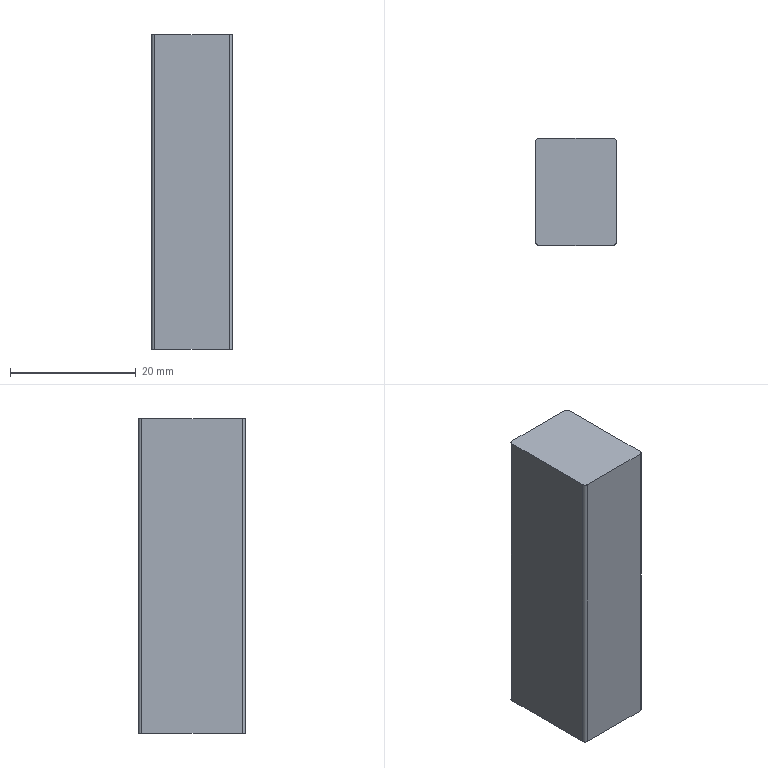Part | NX | features BREP 1 | 1 solid | 10 faces | box 12.887 x 16.955 x 50 mm | volume 10914 mm3 | plane 6 | cylinder 4 | commonest cylinder face diameters 1 x4
STEP:
#1=CARTESIAN_POINT('',(-5.944,8.477,-40.6));
#2=VERTEX_POINT('',#1);
#3=CARTESIAN_POINT('',(-6.444,7.978,-40.6));
#4=VERTEX_POINT('',#3);
#5=CARTESIAN_POINT('',(-5.944,7.978,-40.6));
#6=DIRECTION('',(0.,0.,1.));
#7=DIRECTION('',(1.,0.,0.));
#8=AXIS2_PLACEMENT_3D('',#5,#6,#7);
#9=CIRCLE('',#8,0.5);
#10=EDGE_CURVE('',#2,#4,#9,.T.);
#11=ORIENTED_EDGE('',*,*,#10,.F.);
#12=CARTESIAN_POINT('',(-5.944,8.477,-90.6));
#13=VERTEX_POINT('',#12);
#14=CARTESIAN_POINT('',(-5.944,8.477,-90.6));
#15=DIRECTION('',(0.,0.,1.));
#16=VECTOR('',#15,1000.);
#17=LINE('',#14,#16);
#18=EDGE_CURVE('',#13,#2,#17,.T.);
#19=ORIENTED_EDGE('',*,*,#18,.F.);
#20=CARTESIAN_POINT('',(-6.444,7.978,-90.6));
#21=VERTEX_POINT('',#20);
#22=CARTESIAN_POINT('',(-5.944,7.978,-90.6));
#23=DIRECTION('',(0.,0.,1.));
#24=DIRECTION('',(1.,0.,0.));
#25=AXIS2_PLACEMENT_3D('',#22,#23,#24);
#26=CIRCLE('',#25,0.5);
#27=EDGE_CURVE('',#13,#21,#26,.T.);
#28=ORIENTED_EDGE('',*,*,#27,.T.);
#29=CARTESIAN_POINT('',(-6.444,7.978,-90.6));
#30=DIRECTION('',(0.,0.,1.));
#31=VECTOR('',#30,1000.);
#32=LINE('',#29,#31);
#33=EDGE_CURVE('',#21,#4,#32,.T.);
#34=ORIENTED_EDGE('',*,*,#33,.T.);
#35=EDGE_LOOP('',(#11,#19,#28,#34));
#36=FACE_BOUND('',#35,.T.);
#37=CARTESIAN_POINT('',(-5.944,7.978,-90.6));
#38=DIRECTION('',(0.,0.,1.));
#39=DIRECTION('',(-1.,0.,0.));
#40=AXIS2_PLACEMENT_3D('',#37,#38,#39);
#41=CYLINDRICAL_SURFACE('',#40,0.5);
#42=ADVANCED_FACE('',(#36),#41,.T.);
#43=CARTESIAN_POINT('',(-6.444,-7.977,-40.6));
#44=VERTEX_POINT('',#43);
#45=CARTESIAN_POINT('',(-6.444,-7.977,-40.6));
#46=DIRECTION('',(0.,1.,0.));
#47=VECTOR('',#46,1000.);
#48=LINE('',#45,#47);
#49=EDGE_CURVE('',#44,#4,#48,.T.);
#50=ORIENTED_EDGE('',*,*,#49,.T.);
#51=ORIENTED_EDGE('',*,*,#33,.F.);
#52=CARTESIAN_POINT('',(-6.444,-7.977,-90.6));
#53=VERTEX_POINT('',#52);
#54=CARTESIAN_POINT('',(-6.444,-7.977,-90.6));
#55=DIRECTION('',(0.,1.,0.));
#56=VECTOR('',#55,1000.);
#57=LINE('',#54,#56);
#58=EDGE_CURVE('',#53,#21,#57,.T.);
#59=ORIENTED_EDGE('',*,*,#58,.F.);
#60=CARTESIAN_POINT('',(-6.444,-7.977,-90.6));
#61=DIRECTION('',(0.,0.,1.));
#62=VECTOR('',#61,1000.);
#63=LINE('',#60,#62);
#64=EDGE_CURVE('',#53,#44,#63,.T.);
#65=ORIENTED_EDGE('',*,*,#64,.T.);
#66=EDGE_LOOP('',(#50,#51,#59,#65));
#67=FACE_BOUND('',#66,.T.);
#68=CARTESIAN_POINT('',(-6.444,-7.977,-90.6));
#69=DIRECTION('',(1.,0.,0.));
#70=DIRECTION('',(0.,-1.,0.));
#71=AXIS2_PLACEMENT_3D('',#68,#69,#70);
#72=PLANE('',#71);
#73=ADVANCED_FACE('',(#67),#72,.F.);
#74=CARTESIAN_POINT('',(-5.944,-8.477,-40.6));
#75=VERTEX_POINT('',#74);
#76=CARTESIAN_POINT('',(-5.944,-7.977,-40.6));
#77=DIRECTION('',(0.,0.,1.));
#78=DIRECTION('',(1.,0.,0.));
#79=AXIS2_PLACEMENT_3D('',#76,#77,#78);
#80=CIRCLE('',#79,0.5);
#81=EDGE_CURVE('',#44,#75,#80,.T.);
#82=ORIENTED_EDGE('',*,*,#81,.F.);
#83=ORIENTED_EDGE('',*,*,#64,.F.);
#84=CARTESIAN_POINT('',(-5.944,-8.477,-90.6));
#85=VERTEX_POINT('',#84);
#86=CARTESIAN_POINT('',(-5.944,-7.977,-90.6));
#87=DIRECTION('',(0.,0.,1.));
#88=DIRECTION('',(1.,0.,0.));
#89=AXIS2_PLACEMENT_3D('',#86,#87,#88);
#90=CIRCLE('',#89,0.5);
#91=EDGE_CURVE('',#53,#85,#90,.T.);
#92=ORIENTED_EDGE('',*,*,#91,.T.);
#93=CARTESIAN_POINT('',(-5.944,-8.477,-90.6));
#94=DIRECTION('',(0.,0.,1.));
#95=VECTOR('',#94,1000.);
#96=LINE('',#93,#95);
#97=EDGE_CURVE('',#85,#75,#96,.T.);
#98=ORIENTED_EDGE('',*,*,#97,.T.);
#99=EDGE_LOOP('',(#82,#83,#92,#98));
#100=FACE_BOUND('',#99,.T.);
#101=CARTESIAN_POINT('',(-5.944,-7.977,-90.6));
#102=DIRECTION('',(0.,0.,1.));
#103=DIRECTION('',(-1.,0.,0.));
#104=AXIS2_PLACEMENT_3D('',#101,#102,#103);
#105=CYLINDRICAL_SURFACE('',#104,0.5);
#106=ADVANCED_FACE('',(#100),#105,.T.);
#107=CARTESIAN_POINT('',(5.944,-8.477,-40.6));
#108=VERTEX_POINT('',#107);
#109=CARTESIAN_POINT('',(5.944,-8.477,-40.6));
#110=DIRECTION('',(-1.,0.,0.));
#111=VECTOR('',#110,1000.);
#112=LINE('',#109,#111);
#113=EDGE_CURVE('',#108,#75,#112,.T.);
#114=ORIENTED_EDGE('',*,*,#113,.T.);
#115=ORIENTED_EDGE('',*,*,#97,.F.);
#116=CARTESIAN_POINT('',(5.944,-8.477,-90.6));
#117=VERTEX_POINT('',#116);
#118=CARTESIAN_POINT('',(5.944,-8.477,-90.6));
#119=DIRECTION('',(-1.,0.,0.));
#120=VECTOR('',#119,1000.);
#121=LINE('',#118,#120);
#122=EDGE_CURVE('',#117,#85,#121,.T.);
#123=ORIENTED_EDGE('',*,*,#122,.F.);
#124=CARTESIAN_POINT('',(5.944,-8.477,-90.6));
#125=DIRECTION('',(0.,0.,1.));
#126=VECTOR('',#125,1000.);
#127=LINE('',#124,#126);
#128=EDGE_CURVE('',#117,#108,#127,.T.);
#129=ORIENTED_EDGE('',*,*,#128,.T.);
#130=EDGE_LOOP('',(#114,#115,#123,#129));
#131=FACE_BOUND('',#130,.T.);
#132=CARTESIAN_POINT('',(5.944,-8.477,-90.6));
#133=DIRECTION('',(0.,1.,0.));
#134=DIRECTION('',(0.,0.,-1.));
#135=AXIS2_PLACEMENT_3D('',#132,#133,#134);
#136=PLANE('',#135);
#137=ADVANCED_FACE('',(#131),#136,.F.);
#138=CARTESIAN_POINT('',(6.444,-7.977,-40.6));
#139=VERTEX_POINT('',#138);
#140=CARTESIAN_POINT('',(5.944,-7.977,-40.6));
#141=DIRECTION('',(0.,0.,1.));
#142=DIRECTION('',(1.,0.,0.));
#143=AXIS2_PLACEMENT_3D('',#140,#141,#142);
#144=CIRCLE('',#143,0.5);
#145=EDGE_CURVE('',#108,#139,#144,.T.);
#146=ORIENTED_EDGE('',*,*,#145,.F.);
#147=ORIENTED_EDGE('',*,*,#128,.F.);
#148=CARTESIAN_POINT('',(6.444,-7.977,-90.6));
#149=VERTEX_POINT('',#148);
#150=CARTESIAN_POINT('',(5.944,-7.977,-90.6));
#151=DIRECTION('',(0.,0.,1.));
#152=DIRECTION('',(1.,0.,0.));
#153=AXIS2_PLACEMENT_3D('',#150,#151,#152);
#154=CIRCLE('',#153,0.5);
#155=EDGE_CURVE('',#117,#149,#154,.T.);
#156=ORIENTED_EDGE('',*,*,#155,.T.);
#157=CARTESIAN_POINT('',(6.444,-7.977,-90.6));
#158=DIRECTION('',(0.,0.,1.));
#159=VECTOR('',#158,1000.);
#160=LINE('',#157,#159);
#161=EDGE_CURVE('',#149,#139,#160,.T.);
#162=ORIENTED_EDGE('',*,*,#161,.T.);
#163=EDGE_LOOP('',(#146,#147,#156,#162));
#164=FACE_BOUND('',#163,.T.);
#165=CARTESIAN_POINT('',(5.944,-7.977,-90.6));
#166=DIRECTION('',(0.,0.,1.));
#167=DIRECTION('',(-1.,0.,0.));
#168=AXIS2_PLACEMENT_3D('',#165,#166,#167);
#169=CYLINDRICAL_SURFACE('',#168,0.5);
#170=ADVANCED_FACE('',(#164),#169,.T.);
#171=CARTESIAN_POINT('',(6.444,7.978,-40.6));
#172=VERTEX_POINT('',#171);
#173=CARTESIAN_POINT('',(6.444,7.978,-40.6));
#174=DIRECTION('',(0.,-1.,0.));
#175=VECTOR('',#174,1000.);
#176=LINE('',#173,#175);
#177=EDGE_CURVE('',#172,#139,#176,.T.);
#178=ORIENTED_EDGE('',*,*,#177,.T.);
#179=ORIENTED_EDGE('',*,*,#161,.F.);
#180=CARTESIAN_POINT('',(6.444,7.978,-90.6));
#181=VERTEX_POINT('',#180);
#182=CARTESIAN_POINT('',(6.444,7.978,-90.6));
#183=DIRECTION('',(0.,-1.,0.));
#184=VECTOR('',#183,1000.);
#185=LINE('',#182,#184);
#186=EDGE_CURVE('',#181,#149,#185,.T.);
#187=ORIENTED_EDGE('',*,*,#186,.F.);
#188=CARTESIAN_POINT('',(6.444,7.978,-90.6));
#189=DIRECTION('',(0.,0.,1.));
#190=VECTOR('',#189,1000.);
#191=LINE('',#188,#190);
#192=EDGE_CURVE('',#181,#172,#191,.T.);
#193=ORIENTED_EDGE('',*,*,#192,.T.);
#194=EDGE_LOOP('',(#178,#179,#187,#193));
#195=FACE_BOUND('',#194,.T.);
#196=CARTESIAN_POINT('',(6.444,7.978,-90.6));
#197=DIRECTION('',(-1.,0.,0.));
#198=DIRECTION('',(0.,0.,-1.));
#199=AXIS2_PLACEMENT_3D('',#196,#197,#198);
#200=PLANE('',#199);
#201=ADVANCED_FACE('',(#195),#200,.F.);
#202=CARTESIAN_POINT('',(5.944,8.477,-40.6));
#203=VERTEX_POINT('',#202);
#204=CARTESIAN_POINT('',(5.944,7.978,-40.6));
#205=DIRECTION('',(0.,0.,1.));
#206=DIRECTION('',(1.,0.,0.));
#207=AXIS2_PLACEMENT_3D('',#204,#205,#206);
#208=CIRCLE('',#207,0.5);
#209=EDGE_CURVE('',#172,#203,#208,.T.);
#210=ORIENTED_EDGE('',*,*,#209,.F.);
#211=ORIENTED_EDGE('',*,*,#192,.F.);
#212=CARTESIAN_POINT('',(5.944,8.477,-90.6));
#213=VERTEX_POINT('',#212);
#214=CARTESIAN_POINT('',(5.944,7.978,-90.6));
#215=DIRECTION('',(0.,0.,1.));
#216=DIRECTION('',(1.,0.,0.));
#217=AXIS2_PLACEMENT_3D('',#214,#215,#216);
#218=CIRCLE('',#217,0.5);
#219=EDGE_CURVE('',#181,#213,#218,.T.);
#220=ORIENTED_EDGE('',*,*,#219,.T.);
#221=CARTESIAN_POINT('',(5.944,8.477,-90.6));
#222=DIRECTION('',(0.,0.,1.));
#223=VECTOR('',#222,1000.);
#224=LINE('',#221,#223);
#225=EDGE_CURVE('',#213,#203,#224,.T.);
#226=ORIENTED_EDGE('',*,*,#225,.T.);
#227=EDGE_LOOP('',(#210,#211,#220,#226));
#228=FACE_BOUND('',#227,.T.);
#229=CARTESIAN_POINT('',(5.944,7.978,-90.6));
#230=DIRECTION('',(0.,0.,1.));
#231=DIRECTION('',(-1.,0.,0.));
#232=AXIS2_PLACEMENT_3D('',#229,#230,#231);
#233=CYLINDRICAL_SURFACE('',#232,0.5);
#234=ADVANCED_FACE('',(#228),#233,.T.);
#235=CARTESIAN_POINT('',(-5.944,8.477,-40.6));
#236=DIRECTION('',(1.,0.,0.));
#237=VECTOR('',#236,1000.);
#238=LINE('',#235,#237);
#239=EDGE_CURVE('',#2,#203,#238,.T.);
#240=ORIENTED_EDGE('',*,*,#239,.T.);
#241=ORIENTED_EDGE('',*,*,#225,.F.);
#242=CARTESIAN_POINT('',(-5.944,8.477,-90.6));
#243=DIRECTION('',(1.,0.,0.));
#244=VECTOR('',#243,1000.);
#245=LINE('',#242,#244);
#246=EDGE_CURVE('',#13,#213,#245,.T.);
#247=ORIENTED_EDGE('',*,*,#246,.F.);
#248=ORIENTED_EDGE('',*,*,#18,.T.);
#249=EDGE_LOOP('',(#240,#241,#247,#248));
#250=FACE_BOUND('',#249,.T.);
#251=CARTESIAN_POINT('',(-5.944,8.477,-90.6));
#252=DIRECTION('',(0.,-1.,0.));
#253=DIRECTION('',(-1.,0.,0.));
#254=AXIS2_PLACEMENT_3D('',#251,#252,#253);
#255=PLANE('',#254);
#256=ADVANCED_FACE('',(#250),#255,.F.);
#257=ORIENTED_EDGE('',*,*,#27,.F.);
#258=ORIENTED_EDGE('',*,*,#246,.T.);
#259=ORIENTED_EDGE('',*,*,#219,.F.);
#260=ORIENTED_EDGE('',*,*,#186,.T.);
#261=ORIENTED_EDGE('',*,*,#155,.F.);
#262=ORIENTED_EDGE('',*,*,#122,.T.);
#263=ORIENTED_EDGE('',*,*,#91,.F.);
#264=ORIENTED_EDGE('',*,*,#58,.T.);
#265=EDGE_LOOP('',(#257,#258,#259,#260,#261,#262,#263,#264));
#266=FACE_BOUND('',#265,.T.);
#267=CARTESIAN_POINT('',(-5.944,7.978,-90.6));
#268=DIRECTION('',(0.,0.,1.));
#269=DIRECTION('',(-1.,0.,0.));
#270=AXIS2_PLACEMENT_3D('',#267,#268,#269);
#271=PLANE('',#270);
#272=ADVANCED_FACE('',(#266),#271,.F.);
#273=ORIENTED_EDGE('',*,*,#10,.T.);
#274=ORIENTED_EDGE('',*,*,#49,.F.);
#275=ORIENTED_EDGE('',*,*,#81,.T.);
#276=ORIENTED_EDGE('',*,*,#113,.F.);
#277=ORIENTED_EDGE('',*,*,#145,.T.);
#278=ORIENTED_EDGE('',*,*,#177,.F.);
#279=ORIENTED_EDGE('',*,*,#209,.T.);
#280=ORIENTED_EDGE('',*,*,#239,.F.);
#281=EDGE_LOOP('',(#273,#274,#275,#276,#277,#278,#279,#280));
#282=FACE_BOUND('',#281,.T.);
#283=CARTESIAN_POINT('',(-5.944,7.978,-40.6));
#284=DIRECTION('',(0.,0.,1.));
#285=DIRECTION('',(-1.,0.,0.));
#286=AXIS2_PLACEMENT_3D('',#283,#284,#285);
#287=PLANE('',#286);
#288=ADVANCED_FACE('',(#282),#287,.T.);
#289=CLOSED_SHELL('',(#42,#73,#106,#137,#170,#201,#234,#256,#272,#288));
#290=MANIFOLD_SOLID_BREP('',#289);
#291=(LENGTH_UNIT()NAMED_UNIT(*)SI_UNIT(.MILLI.,.METRE.));
#292=UNCERTAINTY_MEASURE_WITH_UNIT(LENGTH_MEASURE(0.00001),#291,'','');
#293=(NAMED_UNIT(*)PLANE_ANGLE_UNIT()SI_UNIT($,.RADIAN.));
#294=(NAMED_UNIT(*)SI_UNIT($,.STERADIAN.)SOLID_ANGLE_UNIT());
#295=(GEOMETRIC_REPRESENTATION_CONTEXT(3)GLOBAL_UNCERTAINTY_ASSIGNED_CONTEXT((#292))GLOBAL_UNIT_ASSIGNED_CONTEXT((#291,#293,#294))REPRESENTATION_CONTEXT('',''));
#296=ADVANCED_BREP_SHAPE_REPRESENTATION('',(#290),#295);